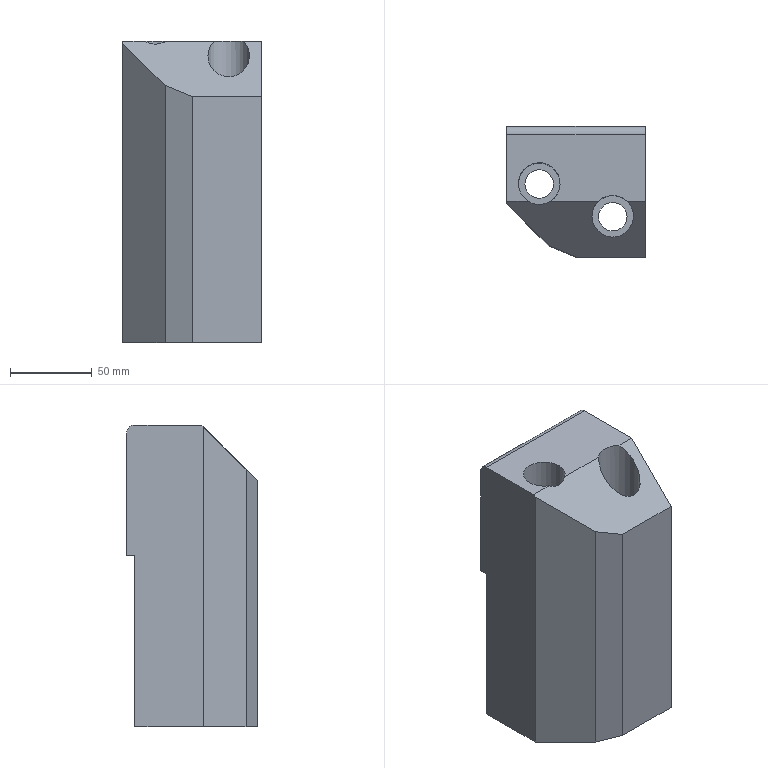Part | NX | features solid 2 | 1 solid | 18 faces | box 85 x 80 x 185 mm | volume 902461 mm3 | plane 13 | cylinder 5 | commonest cylinder face diameters 17.5 x2 25.5 x2 10 x1
STEP:
#1=CARTESIAN_POINT('',(-582.5,-252.071,-180.));
#2=VERTEX_POINT('',#1);
#3=CARTESIAN_POINT('',(-582.5,-252.071,3.787));
#4=VERTEX_POINT('',#3);
#5=CARTESIAN_POINT('',(-582.5,-252.071,-100.));
#6=DIRECTION('',(0.,0.,-1.));
#7=VECTOR('',#6,1000.);
#8=LINE('',#5,#7);
#9=EDGE_CURVE('',#2,#4,#8,.F.);
#10=ORIENTED_EDGE('',*,*,#9,.T.);
#11=CARTESIAN_POINT('',(-582.5,-250.858,5.));
#12=VERTEX_POINT('',#11);
#13=CARTESIAN_POINT('',(-582.5,-257.929,-2.071));
#14=DIRECTION('',(0.,-0.7071,-0.7071));
#15=VECTOR('',#14,1000.);
#16=LINE('',#13,#15);
#17=EDGE_CURVE('',#4,#12,#16,.F.);
#18=ORIENTED_EDGE('',*,*,#17,.T.);
#19=CARTESIAN_POINT('',(-582.5,-210.,5.));
#20=VERTEX_POINT('',#19);
#21=CARTESIAN_POINT('',(-582.5,-205.,5.));
#22=DIRECTION('',(0.,-1.,0.));
#23=VECTOR('',#22,1000.);
#24=LINE('',#21,#23);
#25=EDGE_CURVE('',#20,#12,#24,.T.);
#26=ORIENTED_EDGE('',*,*,#25,.F.);
#27=CARTESIAN_POINT('',(-582.5,-205.,0.));
#28=VERTEX_POINT('',#27);
#29=CARTESIAN_POINT('',(-582.5,-210.,0.));
#30=DIRECTION('',(1.,0.,0.));
#31=DIRECTION('',(0.,0.,-1.));
#32=AXIS2_PLACEMENT_3D('',#29,#30,#31);
#33=CIRCLE('',#32,5.);
#34=EDGE_CURVE('',#20,#28,#33,.F.);
#35=ORIENTED_EDGE('',*,*,#34,.T.);
#36=CARTESIAN_POINT('',(-582.5,-205.,-75.));
#37=VERTEX_POINT('',#36);
#38=CARTESIAN_POINT('',(-582.5,-205.,-100.));
#39=DIRECTION('',(0.,0.,1.));
#40=VECTOR('',#39,1000.);
#41=LINE('',#38,#40);
#42=EDGE_CURVE('',#37,#28,#41,.T.);
#43=ORIENTED_EDGE('',*,*,#42,.F.);
#44=CARTESIAN_POINT('',(-582.5,-210.,-75.));
#45=VERTEX_POINT('',#44);
#46=CARTESIAN_POINT('',(-582.5,-205.,-75.));
#47=DIRECTION('',(0.,1.,0.));
#48=VECTOR('',#47,1000.);
#49=LINE('',#46,#48);
#50=EDGE_CURVE('',#37,#45,#49,.F.);
#51=ORIENTED_EDGE('',*,*,#50,.T.);
#52=CARTESIAN_POINT('',(-582.5,-210.,-180.));
#53=VERTEX_POINT('',#52);
#54=CARTESIAN_POINT('',(-582.5,-210.,-75.));
#55=DIRECTION('',(0.,0.,1.));
#56=VECTOR('',#55,1000.);
#57=LINE('',#54,#56);
#58=EDGE_CURVE('',#45,#53,#57,.F.);
#59=ORIENTED_EDGE('',*,*,#58,.T.);
#60=CARTESIAN_POINT('',(-582.5,-205.,-180.));
#61=DIRECTION('',(0.,-1.,0.));
#62=VECTOR('',#61,1000.);
#63=LINE('',#60,#62);
#64=EDGE_CURVE('',#53,#2,#63,.T.);
#65=ORIENTED_EDGE('',*,*,#64,.T.);
#66=EDGE_LOOP('',(#10,#18,#26,#35,#43,#51,#59,#65));
#67=FACE_BOUND('',#66,.T.);
#68=CARTESIAN_POINT('',(-582.5,-205.,-100.));
#69=DIRECTION('',(1.,0.,0.));
#70=DIRECTION('',(0.,0.,-1.));
#71=AXIS2_PLACEMENT_3D('',#68,#69,#70);
#72=PLANE('',#71);
#73=ADVANCED_FACE('',(#67),#72,.F.);
#74=CARTESIAN_POINT('',(-553.75,-240.,-180.));
#75=VERTEX_POINT('',#74);
#76=CARTESIAN_POINT('',(-562.5,-240.,-180.));
#77=DIRECTION('',(0.,0.,1.));
#78=DIRECTION('',(1.,0.,0.));
#79=AXIS2_PLACEMENT_3D('',#76,#77,#78);
#80=CIRCLE('',#79,8.75);
#81=EDGE_CURVE('',#75,#75,#80,.T.);
#82=ORIENTED_EDGE('',*,*,#81,.T.);
#83=EDGE_LOOP('',(#82));
#84=FACE_BOUND('',#83,.T.);
#85=CARTESIAN_POINT('',(-508.75,-260.,-180.));
#86=VERTEX_POINT('',#85);
#87=CARTESIAN_POINT('',(-517.5,-260.,-180.));
#88=DIRECTION('',(0.,0.,1.));
#89=DIRECTION('',(1.,0.,0.));
#90=AXIS2_PLACEMENT_3D('',#87,#88,#89);
#91=CIRCLE('',#90,8.75);
#92=EDGE_CURVE('',#86,#86,#91,.T.);
#93=ORIENTED_EDGE('',*,*,#92,.T.);
#94=EDGE_LOOP('',(#93));
#95=FACE_BOUND('',#94,.T.);
#96=CARTESIAN_POINT('',(-497.5,-285.,-180.));
#97=VERTEX_POINT('',#96);
#98=CARTESIAN_POINT('',(-539.797,-285.,-180.));
#99=VERTEX_POINT('',#98);
#100=CARTESIAN_POINT('',(-507.5,-285.,-180.));
#101=DIRECTION('',(-1.,0.,0.));
#102=VECTOR('',#101,1000.);
#103=LINE('',#100,#102);
#104=EDGE_CURVE('',#97,#99,#103,.T.);
#105=ORIENTED_EDGE('',*,*,#104,.T.);
#106=CARTESIAN_POINT('',(-556.482,-278.089,-180.));
#107=VERTEX_POINT('',#106);
#108=CARTESIAN_POINT('',(-560.943,-276.241,-180.));
#109=DIRECTION('',(0.9239,-0.3827,0.));
#110=VECTOR('',#109,1000.);
#111=LINE('',#108,#110);
#112=EDGE_CURVE('',#99,#107,#111,.F.);
#113=ORIENTED_EDGE('',*,*,#112,.T.);
#114=CARTESIAN_POINT('',(-586.036,-248.536,-180.));
#115=DIRECTION('',(0.7071,-0.7071,0.));
#116=VECTOR('',#115,1000.);
#117=LINE('',#114,#116);
#118=EDGE_CURVE('',#107,#2,#117,.F.);
#119=ORIENTED_EDGE('',*,*,#118,.T.);
#120=ORIENTED_EDGE('',*,*,#64,.F.);
#121=CARTESIAN_POINT('',(-497.5,-210.,-180.));
#122=VERTEX_POINT('',#121);
#123=CARTESIAN_POINT('',(-507.5,-210.,-180.));
#124=DIRECTION('',(-1.,0.,0.));
#125=VECTOR('',#124,1000.);
#126=LINE('',#123,#125);
#127=EDGE_CURVE('',#122,#53,#126,.T.);
#128=ORIENTED_EDGE('',*,*,#127,.F.);
#129=CARTESIAN_POINT('',(-497.5,-205.,-180.));
#130=DIRECTION('',(0.,-1.,0.));
#131=VECTOR('',#130,1000.);
#132=LINE('',#129,#131);
#133=EDGE_CURVE('',#122,#97,#132,.T.);
#134=ORIENTED_EDGE('',*,*,#133,.T.);
#135=EDGE_LOOP('',(#105,#113,#119,#120,#128,#134));
#136=FACE_BOUND('',#135,.T.);
#137=CARTESIAN_POINT('',(-507.5,-205.,-180.));
#138=DIRECTION('',(0.,0.,1.));
#139=DIRECTION('',(1.,0.,0.));
#140=AXIS2_PLACEMENT_3D('',#137,#138,#139);
#141=PLANE('',#140);
#142=ADVANCED_FACE('',(#84,#95,#136),#141,.F.);
#143=CARTESIAN_POINT('',(-497.5,-210.,5.));
#144=VERTEX_POINT('',#143);
#145=CARTESIAN_POINT('',(-497.5,-250.858,5.));
#146=VERTEX_POINT('',#145);
#147=CARTESIAN_POINT('',(-497.5,-205.,5.));
#148=DIRECTION('',(0.,-1.,0.));
#149=VECTOR('',#148,1000.);
#150=LINE('',#147,#149);
#151=EDGE_CURVE('',#144,#146,#150,.T.);
#152=ORIENTED_EDGE('',*,*,#151,.T.);
#153=CARTESIAN_POINT('',(-497.5,-285.,-29.142));
#154=VERTEX_POINT('',#153);
#155=CARTESIAN_POINT('',(-497.5,-257.929,-2.071));
#156=DIRECTION('',(0.,0.7071,0.7071));
#157=VECTOR('',#156,1000.);
#158=LINE('',#155,#157);
#159=EDGE_CURVE('',#146,#154,#158,.F.);
#160=ORIENTED_EDGE('',*,*,#159,.T.);
#161=CARTESIAN_POINT('',(-497.5,-285.,0.));
#162=DIRECTION('',(0.,0.,-1.));
#163=VECTOR('',#162,1000.);
#164=LINE('',#161,#163);
#165=EDGE_CURVE('',#154,#97,#164,.T.);
#166=ORIENTED_EDGE('',*,*,#165,.T.);
#167=ORIENTED_EDGE('',*,*,#133,.F.);
#168=CARTESIAN_POINT('',(-497.5,-210.,-75.));
#169=VERTEX_POINT('',#168);
#170=CARTESIAN_POINT('',(-497.5,-210.,-75.));
#171=DIRECTION('',(0.,0.,1.));
#172=VECTOR('',#171,1000.);
#173=LINE('',#170,#172);
#174=EDGE_CURVE('',#169,#122,#173,.F.);
#175=ORIENTED_EDGE('',*,*,#174,.F.);
#176=CARTESIAN_POINT('',(-497.5,-205.,-75.));
#177=VERTEX_POINT('',#176);
#178=CARTESIAN_POINT('',(-497.5,-205.,-75.));
#179=DIRECTION('',(0.,1.,0.));
#180=VECTOR('',#179,1000.);
#181=LINE('',#178,#180);
#182=EDGE_CURVE('',#177,#169,#181,.F.);
#183=ORIENTED_EDGE('',*,*,#182,.F.);
#184=CARTESIAN_POINT('',(-497.5,-205.,0.));
#185=VERTEX_POINT('',#184);
#186=CARTESIAN_POINT('',(-497.5,-205.,0.));
#187=DIRECTION('',(0.,0.,-1.));
#188=VECTOR('',#187,1000.);
#189=LINE('',#186,#188);
#190=EDGE_CURVE('',#185,#177,#189,.T.);
#191=ORIENTED_EDGE('',*,*,#190,.F.);
#192=CARTESIAN_POINT('',(-497.5,-210.,0.));
#193=DIRECTION('',(-1.,0.,0.));
#194=DIRECTION('',(0.,0.,1.));
#195=AXIS2_PLACEMENT_3D('',#192,#193,#194);
#196=CIRCLE('',#195,5.);
#197=EDGE_CURVE('',#185,#144,#196,.F.);
#198=ORIENTED_EDGE('',*,*,#197,.T.);
#199=EDGE_LOOP('',(#152,#160,#166,#167,#175,#183,#191,#198));
#200=FACE_BOUND('',#199,.T.);
#201=CARTESIAN_POINT('',(-497.5,-205.,0.));
#202=DIRECTION('',(-1.,0.,0.));
#203=DIRECTION('',(0.,0.,1.));
#204=AXIS2_PLACEMENT_3D('',#201,#202,#203);
#205=PLANE('',#204);
#206=ADVANCED_FACE('',(#200),#205,.F.);
#207=ORIENTED_EDGE('',*,*,#42,.T.);
#208=CARTESIAN_POINT('',(-497.5,-205.,0.));
#209=DIRECTION('',(1.,0.,0.));
#210=VECTOR('',#209,1000.);
#211=LINE('',#208,#210);
#212=EDGE_CURVE('',#28,#185,#211,.T.);
#213=ORIENTED_EDGE('',*,*,#212,.T.);
#214=ORIENTED_EDGE('',*,*,#190,.T.);
#215=CARTESIAN_POINT('',(-507.5,-205.,-75.));
#216=DIRECTION('',(1.,0.,0.));
#217=VECTOR('',#216,1000.);
#218=LINE('',#215,#217);
#219=EDGE_CURVE('',#177,#37,#218,.F.);
#220=ORIENTED_EDGE('',*,*,#219,.T.);
#221=EDGE_LOOP('',(#207,#213,#214,#220));
#222=FACE_BOUND('',#221,.T.);
#223=CARTESIAN_POINT('',(-507.5,-205.,0.));
#224=DIRECTION('',(0.,1.,0.));
#225=DIRECTION('',(-1.,0.,0.));
#226=AXIS2_PLACEMENT_3D('',#223,#224,#225);
#227=PLANE('',#226);
#228=ADVANCED_FACE('',(#222),#227,.T.);
#229=ORIENTED_EDGE('',*,*,#25,.T.);
#230=CARTESIAN_POINT('',(-569.184,-250.858,5.));
#231=VERTEX_POINT('',#230);
#232=CARTESIAN_POINT('',(-582.5,-250.858,5.));
#233=DIRECTION('',(-1.,0.,0.));
#234=VECTOR('',#233,1000.);
#235=LINE('',#232,#234);
#236=EDGE_CURVE('',#12,#231,#235,.F.);
#237=ORIENTED_EDGE('',*,*,#236,.T.);
#238=CARTESIAN_POINT('',(-555.816,-250.858,5.));
#239=VERTEX_POINT('',#238);
#240=CARTESIAN_POINT('',(-562.5,-240.,5.));
#241=DIRECTION('',(0.,0.,-1.));
#242=DIRECTION('',(-1.,0.,0.));
#243=AXIS2_PLACEMENT_3D('',#240,#241,#242);
#244=CIRCLE('',#243,12.75);
#245=EDGE_CURVE('',#231,#239,#244,.T.);
#246=ORIENTED_EDGE('',*,*,#245,.T.);
#247=CARTESIAN_POINT('',(-526.387,-250.858,5.));
#248=VERTEX_POINT('',#247);
#249=CARTESIAN_POINT('',(-582.5,-250.858,5.));
#250=DIRECTION('',(-1.,0.,0.));
#251=VECTOR('',#250,1000.);
#252=LINE('',#249,#251);
#253=EDGE_CURVE('',#239,#248,#252,.F.);
#254=ORIENTED_EDGE('',*,*,#253,.T.);
#255=CARTESIAN_POINT('',(-508.613,-250.858,5.));
#256=VERTEX_POINT('',#255);
#257=CARTESIAN_POINT('',(-517.5,-260.,5.));
#258=DIRECTION('',(0.,0.,-1.));
#259=DIRECTION('',(-1.,0.,0.));
#260=AXIS2_PLACEMENT_3D('',#257,#258,#259);
#261=CIRCLE('',#260,12.75);
#262=EDGE_CURVE('',#248,#256,#261,.T.);
#263=ORIENTED_EDGE('',*,*,#262,.T.);
#264=CARTESIAN_POINT('',(-582.5,-250.858,5.));
#265=DIRECTION('',(-1.,0.,0.));
#266=VECTOR('',#265,1000.);
#267=LINE('',#264,#266);
#268=EDGE_CURVE('',#256,#146,#267,.F.);
#269=ORIENTED_EDGE('',*,*,#268,.T.);
#270=ORIENTED_EDGE('',*,*,#151,.F.);
#271=CARTESIAN_POINT('',(-582.5,-210.,5.));
#272=DIRECTION('',(1.,0.,0.));
#273=VECTOR('',#272,1000.);
#274=LINE('',#271,#273);
#275=EDGE_CURVE('',#144,#20,#274,.F.);
#276=ORIENTED_EDGE('',*,*,#275,.T.);
#277=EDGE_LOOP('',(#229,#237,#246,#254,#263,#269,#270,#276));
#278=FACE_BOUND('',#277,.T.);
#279=CARTESIAN_POINT('',(-582.5,-205.,5.));
#280=DIRECTION('',(0.,0.,-1.));
#281=DIRECTION('',(-1.,0.,0.));
#282=AXIS2_PLACEMENT_3D('',#279,#280,#281);
#283=PLANE('',#282);
#284=ADVANCED_FACE('',(#278),#283,.F.);
#285=ORIENTED_EDGE('',*,*,#165,.F.);
#286=CARTESIAN_POINT('',(-539.797,-285.,-29.142));
#287=VERTEX_POINT('',#286);
#288=CARTESIAN_POINT('',(-582.5,-285.,-29.142));
#289=DIRECTION('',(1.,0.,0.));
#290=VECTOR('',#289,1000.);
#291=LINE('',#288,#290);
#292=EDGE_CURVE('',#154,#287,#291,.F.);
#293=ORIENTED_EDGE('',*,*,#292,.T.);
#294=CARTESIAN_POINT('',(-539.797,-285.,-100.));
#295=DIRECTION('',(0.,0.,1.));
#296=VECTOR('',#295,1000.);
#297=LINE('',#294,#296);
#298=EDGE_CURVE('',#287,#99,#297,.F.);
#299=ORIENTED_EDGE('',*,*,#298,.T.);
#300=ORIENTED_EDGE('',*,*,#104,.F.);
#301=EDGE_LOOP('',(#285,#293,#299,#300));
#302=FACE_BOUND('',#301,.T.);
#303=CARTESIAN_POINT('',(-507.5,-285.,0.));
#304=DIRECTION('',(0.,1.,0.));
#305=DIRECTION('',(-1.,0.,0.));
#306=AXIS2_PLACEMENT_3D('',#303,#304,#305);
#307=PLANE('',#306);
#308=ADVANCED_FACE('',(#302),#307,.F.);
#309=CARTESIAN_POINT('',(-556.482,-278.089,-22.231));
#310=VERTEX_POINT('',#309);
#311=CARTESIAN_POINT('',(-556.482,-278.089,-100.));
#312=DIRECTION('',(0.,0.,1.));
#313=VECTOR('',#312,1000.);
#314=LINE('',#311,#313);
#315=EDGE_CURVE('',#107,#310,#314,.T.);
#316=ORIENTED_EDGE('',*,*,#315,.T.);
#317=CARTESIAN_POINT('',(-550.261,-284.31,-28.452));
#318=DIRECTION('',(-0.5774,0.5774,0.5774));
#319=VECTOR('',#318,1000.);
#320=LINE('',#317,#319);
#321=EDGE_CURVE('',#310,#4,#320,.T.);
#322=ORIENTED_EDGE('',*,*,#321,.T.);
#323=ORIENTED_EDGE('',*,*,#9,.F.);
#324=ORIENTED_EDGE('',*,*,#118,.F.);
#325=EDGE_LOOP('',(#316,#322,#323,#324));
#326=FACE_BOUND('',#325,.T.);
#327=CARTESIAN_POINT('',(-586.036,-248.536,-100.));
#328=DIRECTION('',(0.7071,0.7071,0.));
#329=DIRECTION('',(-0.7071,0.7071,0.));
#330=AXIS2_PLACEMENT_3D('',#327,#328,#329);
#331=PLANE('',#330);
#332=ADVANCED_FACE('',(#326),#331,.F.);
#333=CARTESIAN_POINT('',(-571.25,-240.,-150.));
#334=VERTEX_POINT('',#333);
#335=CARTESIAN_POINT('',(-562.5,-240.,-150.));
#336=DIRECTION('',(0.,0.,-1.));
#337=DIRECTION('',(-1.,0.,0.));
#338=AXIS2_PLACEMENT_3D('',#335,#336,#337);
#339=CIRCLE('',#338,8.75);
#340=EDGE_CURVE('',#334,#334,#339,.T.);
#341=ORIENTED_EDGE('',*,*,#340,.F.);
#342=EDGE_LOOP('',(#341));
#343=FACE_BOUND('',#342,.T.);
#344=ORIENTED_EDGE('',*,*,#81,.F.);
#345=EDGE_LOOP('',(#344));
#346=FACE_BOUND('',#345,.T.);
#347=CARTESIAN_POINT('',(-562.5,-240.,-200.));
#348=DIRECTION('',(0.,0.,-1.));
#349=DIRECTION('',(-1.,0.,0.));
#350=AXIS2_PLACEMENT_3D('',#347,#348,#349);
#351=CYLINDRICAL_SURFACE('',#350,8.75);
#352=ADVANCED_FACE('',(#343,#346),#351,.F.);
#353=ORIENTED_EDGE('',*,*,#340,.T.);
#354=EDGE_LOOP('',(#353));
#355=FACE_BOUND('',#354,.T.);
#356=CARTESIAN_POINT('',(-575.25,-240.,-150.));
#357=VERTEX_POINT('',#356);
#358=CARTESIAN_POINT('',(-562.5,-240.,-150.));
#359=DIRECTION('',(0.,0.,-1.));
#360=DIRECTION('',(-1.,0.,0.));
#361=AXIS2_PLACEMENT_3D('',#358,#359,#360);
#362=CIRCLE('',#361,12.75);
#363=EDGE_CURVE('',#357,#357,#362,.T.);
#364=ORIENTED_EDGE('',*,*,#363,.F.);
#365=EDGE_LOOP('',(#364));
#366=FACE_BOUND('',#365,.T.);
#367=CARTESIAN_POINT('',(-562.5,-225.,-150.));
#368=DIRECTION('',(0.,0.,-1.));
#369=DIRECTION('',(-1.,0.,0.));
#370=AXIS2_PLACEMENT_3D('',#367,#368,#369);
#371=PLANE('',#370);
#372=ADVANCED_FACE('',(#355,#366),#371,.F.);
#373=CARTESIAN_POINT('',(-562.5,-240.,15.858));
#374=DIRECTION('',(0.,0.7071,-0.7071));
#375=DIRECTION('',(0.,-0.7071,-0.7071));
#376=AXIS2_PLACEMENT_3D('',#373,#374,#375);
#377=ELLIPSE('',#376,18.031,12.75);
#378=EDGE_CURVE('',#239,#231,#377,.T.);
#379=ORIENTED_EDGE('',*,*,#378,.F.);
#380=ORIENTED_EDGE('',*,*,#245,.F.);
#381=EDGE_LOOP('',(#379,#380));
#382=FACE_BOUND('',#381,.T.);
#383=ORIENTED_EDGE('',*,*,#363,.T.);
#384=EDGE_LOOP('',(#383));
#385=FACE_BOUND('',#384,.T.);
#386=CARTESIAN_POINT('',(-562.5,-240.,0.));
#387=DIRECTION('',(0.,0.,-1.));
#388=DIRECTION('',(-1.,0.,0.));
#389=AXIS2_PLACEMENT_3D('',#386,#387,#388);
#390=CYLINDRICAL_SURFACE('',#389,12.75);
#391=ADVANCED_FACE('',(#382,#385),#390,.F.);
#392=CARTESIAN_POINT('',(-526.25,-260.,-150.));
#393=VERTEX_POINT('',#392);
#394=CARTESIAN_POINT('',(-517.5,-260.,-150.));
#395=DIRECTION('',(0.,0.,-1.));
#396=DIRECTION('',(-1.,0.,0.));
#397=AXIS2_PLACEMENT_3D('',#394,#395,#396);
#398=CIRCLE('',#397,8.75);
#399=EDGE_CURVE('',#393,#393,#398,.T.);
#400=ORIENTED_EDGE('',*,*,#399,.F.);
#401=EDGE_LOOP('',(#400));
#402=FACE_BOUND('',#401,.T.);
#403=ORIENTED_EDGE('',*,*,#92,.F.);
#404=EDGE_LOOP('',(#403));
#405=FACE_BOUND('',#404,.T.);
#406=CARTESIAN_POINT('',(-517.5,-260.,-200.));
#407=DIRECTION('',(0.,0.,-1.));
#408=DIRECTION('',(-1.,0.,0.));
#409=AXIS2_PLACEMENT_3D('',#406,#407,#408);
#410=CYLINDRICAL_SURFACE('',#409,8.75);
#411=ADVANCED_FACE('',(#402,#405),#410,.F.);
#412=ORIENTED_EDGE('',*,*,#399,.T.);
#413=EDGE_LOOP('',(#412));
#414=FACE_BOUND('',#413,.T.);
#415=CARTESIAN_POINT('',(-530.25,-260.,-150.));
#416=VERTEX_POINT('',#415);
#417=CARTESIAN_POINT('',(-517.5,-260.,-150.));
#418=DIRECTION('',(0.,0.,-1.));
#419=DIRECTION('',(-1.,0.,0.));
#420=AXIS2_PLACEMENT_3D('',#417,#418,#419);
#421=CIRCLE('',#420,12.75);
#422=EDGE_CURVE('',#416,#416,#421,.T.);
#423=ORIENTED_EDGE('',*,*,#422,.F.);
#424=EDGE_LOOP('',(#423));
#425=FACE_BOUND('',#424,.T.);
#426=CARTESIAN_POINT('',(-527.5,-250.,-150.));
#427=DIRECTION('',(0.,0.,-1.));
#428=DIRECTION('',(-1.,0.,0.));
#429=AXIS2_PLACEMENT_3D('',#426,#427,#428);
#430=PLANE('',#429);
#431=ADVANCED_FACE('',(#414,#425),#430,.F.);
#432=ORIENTED_EDGE('',*,*,#422,.T.);
#433=EDGE_LOOP('',(#432));
#434=FACE_BOUND('',#433,.T.);
#435=ORIENTED_EDGE('',*,*,#262,.F.);
#436=CARTESIAN_POINT('',(-517.5,-260.,-4.142));
#437=DIRECTION('',(0.,0.7071,-0.7071));
#438=DIRECTION('',(0.,-0.7071,-0.7071));
#439=AXIS2_PLACEMENT_3D('',#436,#437,#438);
#440=ELLIPSE('',#439,18.031,12.75);
#441=EDGE_CURVE('',#248,#256,#440,.F.);
#442=ORIENTED_EDGE('',*,*,#441,.T.);
#443=EDGE_LOOP('',(#435,#442));
#444=FACE_BOUND('',#443,.T.);
#445=CARTESIAN_POINT('',(-517.5,-260.,0.));
#446=DIRECTION('',(0.,0.,-1.));
#447=DIRECTION('',(-1.,0.,0.));
#448=AXIS2_PLACEMENT_3D('',#445,#446,#447);
#449=CYLINDRICAL_SURFACE('',#448,12.75);
#450=ADVANCED_FACE('',(#434,#444),#449,.F.);
#451=ORIENTED_EDGE('',*,*,#127,.T.);
#452=ORIENTED_EDGE('',*,*,#58,.F.);
#453=CARTESIAN_POINT('',(-582.5,-210.,-75.));
#454=DIRECTION('',(1.,0.,0.));
#455=VECTOR('',#454,1000.);
#456=LINE('',#453,#455);
#457=EDGE_CURVE('',#45,#169,#456,.T.);
#458=ORIENTED_EDGE('',*,*,#457,.T.);
#459=ORIENTED_EDGE('',*,*,#174,.T.);
#460=EDGE_LOOP('',(#451,#452,#458,#459));
#461=FACE_BOUND('',#460,.T.);
#462=CARTESIAN_POINT('',(-582.5,-210.,-75.));
#463=DIRECTION('',(0.,1.,0.));
#464=DIRECTION('',(0.,0.,1.));
#465=AXIS2_PLACEMENT_3D('',#462,#463,#464);
#466=PLANE('',#465);
#467=ADVANCED_FACE('',(#461),#466,.T.);
#468=ORIENTED_EDGE('',*,*,#182,.T.);
#469=ORIENTED_EDGE('',*,*,#457,.F.);
#470=ORIENTED_EDGE('',*,*,#50,.F.);
#471=ORIENTED_EDGE('',*,*,#219,.F.);
#472=EDGE_LOOP('',(#468,#469,#470,#471));
#473=FACE_BOUND('',#472,.T.);
#474=CARTESIAN_POINT('',(-582.5,-205.,-75.));
#475=DIRECTION('',(0.,0.,1.));
#476=DIRECTION('',(1.,0.,0.));
#477=AXIS2_PLACEMENT_3D('',#474,#475,#476);
#478=PLANE('',#477);
#479=ADVANCED_FACE('',(#473),#478,.F.);
#480=ORIENTED_EDGE('',*,*,#34,.F.);
#481=ORIENTED_EDGE('',*,*,#275,.F.);
#482=ORIENTED_EDGE('',*,*,#197,.F.);
#483=ORIENTED_EDGE('',*,*,#212,.F.);
#484=EDGE_LOOP('',(#480,#481,#482,#483));
#485=FACE_BOUND('',#484,.T.);
#486=CARTESIAN_POINT('',(-507.5,-210.,0.));
#487=DIRECTION('',(-1.,0.,0.));
#488=DIRECTION('',(0.,0.,1.));
#489=AXIS2_PLACEMENT_3D('',#486,#487,#488);
#490=CYLINDRICAL_SURFACE('',#489,5.);
#491=ADVANCED_FACE('',(#485),#490,.T.);
#492=ORIENTED_EDGE('',*,*,#298,.F.);
#493=CARTESIAN_POINT('',(-536.39,-286.411,-30.553));
#494=DIRECTION('',(-0.8629,0.3574,0.3574));
#495=VECTOR('',#494,1000.);
#496=LINE('',#493,#495);
#497=EDGE_CURVE('',#287,#310,#496,.T.);
#498=ORIENTED_EDGE('',*,*,#497,.T.);
#499=ORIENTED_EDGE('',*,*,#315,.F.);
#500=ORIENTED_EDGE('',*,*,#112,.F.);
#501=EDGE_LOOP('',(#492,#498,#499,#500));
#502=FACE_BOUND('',#501,.T.);
#503=CARTESIAN_POINT('',(-560.943,-276.241,-100.));
#504=DIRECTION('',(0.3827,0.9239,0.));
#505=DIRECTION('',(-0.9239,0.3827,0.));
#506=AXIS2_PLACEMENT_3D('',#503,#504,#505);
#507=PLANE('',#506);
#508=ADVANCED_FACE('',(#502),#507,.F.);
#509=ORIENTED_EDGE('',*,*,#253,.F.);
#510=ORIENTED_EDGE('',*,*,#378,.T.);
#511=ORIENTED_EDGE('',*,*,#236,.F.);
#512=ORIENTED_EDGE('',*,*,#17,.F.);
#513=ORIENTED_EDGE('',*,*,#321,.F.);
#514=ORIENTED_EDGE('',*,*,#497,.F.);
#515=ORIENTED_EDGE('',*,*,#292,.F.);
#516=ORIENTED_EDGE('',*,*,#159,.F.);
#517=ORIENTED_EDGE('',*,*,#268,.F.);
#518=ORIENTED_EDGE('',*,*,#441,.F.);
#519=EDGE_LOOP('',(#509,#510,#511,#512,#513,#514,#515,#516,#517,#518));
#520=FACE_BOUND('',#519,.T.);
#521=CARTESIAN_POINT('',(-582.5,-257.929,-2.071));
#522=DIRECTION('',(0.,0.7071,-0.7071));
#523=DIRECTION('',(0.,0.7071,0.7071));
#524=AXIS2_PLACEMENT_3D('',#521,#522,#523);
#525=PLANE('',#524);
#526=ADVANCED_FACE('',(#520),#525,.F.);
#527=CLOSED_SHELL('',(#73,#142,#206,#228,#284,#308,#332,#352,#372,#391,#411,#431,#450,#467,#479,#491,#508,#526));
#528=MANIFOLD_SOLID_BREP('',#527);
#529=(LENGTH_UNIT()NAMED_UNIT(*)SI_UNIT(.MILLI.,.METRE.));
#530=UNCERTAINTY_MEASURE_WITH_UNIT(LENGTH_MEASURE(0.00001),#529,'','');
#531=(NAMED_UNIT(*)PLANE_ANGLE_UNIT()SI_UNIT($,.RADIAN.));
#532=(NAMED_UNIT(*)SI_UNIT($,.STERADIAN.)SOLID_ANGLE_UNIT());
#533=(GEOMETRIC_REPRESENTATION_CONTEXT(3)GLOBAL_UNCERTAINTY_ASSIGNED_CONTEXT((#530))GLOBAL_UNIT_ASSIGNED_CONTEXT((#529,#531,#532))REPRESENTATION_CONTEXT('',''));
#534=ADVANCED_BREP_SHAPE_REPRESENTATION('',(#528),#533);